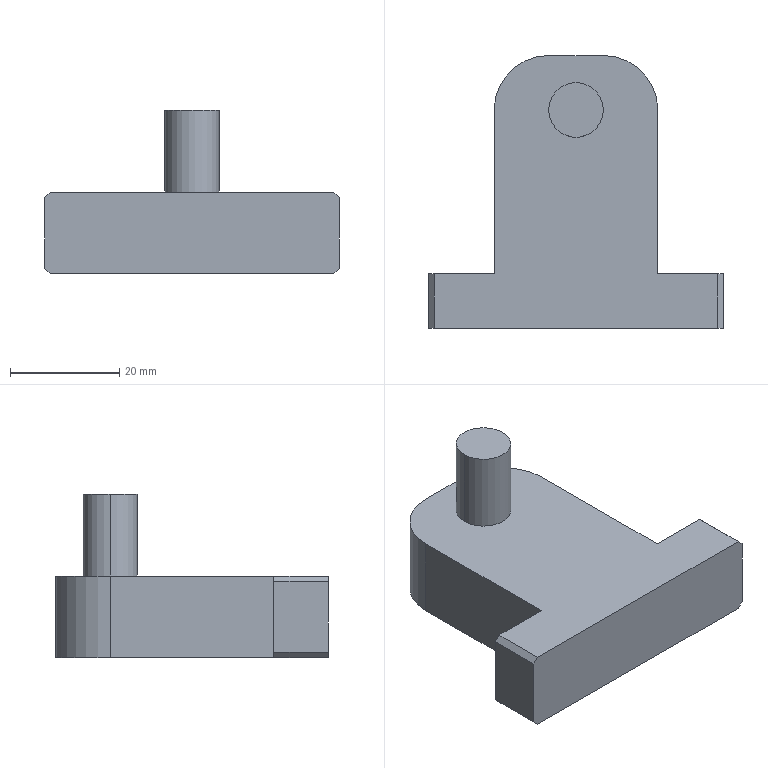Part | SolidWorks | 1 solid | 19 faces | box 54 x 50 x 30 mm | volume 26614 mm3 | plane 15 | cylinder 4 | commonest cylinder face diameters 10 x2 20 x2
STEP:
#1=CARTESIAN_POINT('',(5.,35.,30.));
#2=VERTEX_POINT('',#1);
#3=CARTESIAN_POINT('',(-5.,35.,30.));
#4=VERTEX_POINT('',#3);
#5=CARTESIAN_POINT('',(0.,35.,30.));
#6=DIRECTION('',(0.,0.,1.));
#7=DIRECTION('',(1.,0.,0.));
#8=AXIS2_PLACEMENT_3D('',#5,#6,#7);
#9=CIRCLE('',#8,5.);
#10=EDGE_CURVE('',#2,#4,#9,.T.);
#11=ORIENTED_EDGE('',*,*,#10,.F.);
#12=CARTESIAN_POINT('',(5.,35.,15.));
#13=VERTEX_POINT('',#12);
#14=CARTESIAN_POINT('',(5.,35.,30.));
#15=DIRECTION('',(0.,0.,-1.));
#16=VECTOR('',#15,1000.);
#17=LINE('',#14,#16);
#18=EDGE_CURVE('',#2,#13,#17,.T.);
#19=ORIENTED_EDGE('',*,*,#18,.T.);
#20=CARTESIAN_POINT('',(-5.,35.,15.));
#21=VERTEX_POINT('',#20);
#22=CARTESIAN_POINT('',(0.,35.,15.));
#23=DIRECTION('',(0.,0.,1.));
#24=DIRECTION('',(1.,0.,0.));
#25=AXIS2_PLACEMENT_3D('',#22,#23,#24);
#26=CIRCLE('',#25,5.);
#27=EDGE_CURVE('',#13,#21,#26,.T.);
#28=ORIENTED_EDGE('',*,*,#27,.T.);
#29=CARTESIAN_POINT('',(-5.,35.,30.));
#30=DIRECTION('',(0.,0.,-1.));
#31=VECTOR('',#30,1000.);
#32=LINE('',#29,#31);
#33=EDGE_CURVE('',#4,#21,#32,.T.);
#34=ORIENTED_EDGE('',*,*,#33,.F.);
#35=EDGE_LOOP('',(#11,#19,#28,#34));
#36=FACE_OUTER_BOUND('',#35,.T.);
#37=CARTESIAN_POINT('',(0.,35.,30.));
#38=DIRECTION('',(0.,0.,-1.));
#39=DIRECTION('',(-1.,0.,0.));
#40=AXIS2_PLACEMENT_3D('',#37,#38,#39);
#41=CYLINDRICAL_SURFACE('',#40,5.);
#42=ADVANCED_FACE('',(#36),#41,.T.);
#43=CARTESIAN_POINT('',(27.,-5.,14.));
#44=VERTEX_POINT('',#43);
#45=CARTESIAN_POINT('',(27.,-5.,1.));
#46=VERTEX_POINT('',#45);
#47=CARTESIAN_POINT('',(27.,-5.,15.));
#48=DIRECTION('',(0.,0.,-1.));
#49=VECTOR('',#48,1000.);
#50=LINE('',#47,#49);
#51=EDGE_CURVE('',#44,#46,#50,.T.);
#52=ORIENTED_EDGE('',*,*,#51,.T.);
#53=CARTESIAN_POINT('',(27.,5.,1.));
#54=VERTEX_POINT('',#53);
#55=CARTESIAN_POINT('',(27.,5.,1.));
#56=DIRECTION('',(0.,1.,0.));
#57=VECTOR('',#56,1000.);
#58=LINE('',#55,#57);
#59=EDGE_CURVE('',#46,#54,#58,.T.);
#60=ORIENTED_EDGE('',*,*,#59,.T.);
#61=CARTESIAN_POINT('',(27.,5.,14.));
#62=VERTEX_POINT('',#61);
#63=CARTESIAN_POINT('',(27.,5.,15.));
#64=DIRECTION('',(0.,0.,-1.));
#65=VECTOR('',#64,1000.);
#66=LINE('',#63,#65);
#67=EDGE_CURVE('',#62,#54,#66,.T.);
#68=ORIENTED_EDGE('',*,*,#67,.F.);
#69=CARTESIAN_POINT('',(27.,-5.,14.));
#70=DIRECTION('',(0.,-1.,0.));
#71=VECTOR('',#70,1000.);
#72=LINE('',#69,#71);
#73=EDGE_CURVE('',#62,#44,#72,.T.);
#74=ORIENTED_EDGE('',*,*,#73,.T.);
#75=EDGE_LOOP('',(#52,#60,#68,#74));
#76=FACE_OUTER_BOUND('',#75,.T.);
#77=CARTESIAN_POINT('',(27.,5.,15.));
#78=DIRECTION('',(-1.,0.,0.));
#79=DIRECTION('',(0.,-1.,0.));
#80=AXIS2_PLACEMENT_3D('',#77,#78,#79);
#81=PLANE('',#80);
#82=ADVANCED_FACE('',(#76),#81,.F.);
#83=ORIENTED_EDGE('',*,*,#67,.T.);
#84=CARTESIAN_POINT('',(26.,5.,0.));
#85=VERTEX_POINT('',#84);
#86=CARTESIAN_POINT('',(27.,5.,1.));
#87=DIRECTION('',(-0.7071,0.,-0.7071));
#88=VECTOR('',#87,1000.);
#89=LINE('',#86,#88);
#90=EDGE_CURVE('',#54,#85,#89,.T.);
#91=ORIENTED_EDGE('',*,*,#90,.T.);
#92=CARTESIAN_POINT('',(15.,5.,0.));
#93=VERTEX_POINT('',#92);
#94=CARTESIAN_POINT('',(15.,5.,0.));
#95=DIRECTION('',(-1.,0.,0.));
#96=VECTOR('',#95,1000.);
#97=LINE('',#94,#96);
#98=EDGE_CURVE('',#85,#93,#97,.T.);
#99=ORIENTED_EDGE('',*,*,#98,.T.);
#100=CARTESIAN_POINT('',(15.,5.,15.));
#101=VERTEX_POINT('',#100);
#102=CARTESIAN_POINT('',(15.,5.,15.));
#103=DIRECTION('',(0.,0.,-1.));
#104=VECTOR('',#103,1000.);
#105=LINE('',#102,#104);
#106=EDGE_CURVE('',#101,#93,#105,.T.);
#107=ORIENTED_EDGE('',*,*,#106,.F.);
#108=CARTESIAN_POINT('',(26.,5.,15.));
#109=VERTEX_POINT('',#108);
#110=CARTESIAN_POINT('',(15.,5.,15.));
#111=DIRECTION('',(-1.,0.,0.));
#112=VECTOR('',#111,1000.);
#113=LINE('',#110,#112);
#114=EDGE_CURVE('',#109,#101,#113,.T.);
#115=ORIENTED_EDGE('',*,*,#114,.F.);
#116=CARTESIAN_POINT('',(26.,5.,15.));
#117=DIRECTION('',(0.7071,0.,-0.7071));
#118=VECTOR('',#117,1000.);
#119=LINE('',#116,#118);
#120=EDGE_CURVE('',#109,#62,#119,.T.);
#121=ORIENTED_EDGE('',*,*,#120,.T.);
#122=EDGE_LOOP('',(#83,#91,#99,#107,#115,#121));
#123=FACE_OUTER_BOUND('',#122,.T.);
#124=CARTESIAN_POINT('',(15.,5.,15.));
#125=DIRECTION('',(0.,-1.,0.));
#126=DIRECTION('',(0.,0.,-1.));
#127=AXIS2_PLACEMENT_3D('',#124,#125,#126);
#128=PLANE('',#127);
#129=ADVANCED_FACE('',(#123),#128,.F.);
#130=CARTESIAN_POINT('',(15.,35.,0.));
#131=VERTEX_POINT('',#130);
#132=CARTESIAN_POINT('',(15.,5.,0.));
#133=DIRECTION('',(0.,1.,0.));
#134=VECTOR('',#133,1000.);
#135=LINE('',#132,#134);
#136=EDGE_CURVE('',#93,#131,#135,.T.);
#137=ORIENTED_EDGE('',*,*,#136,.T.);
#138=CARTESIAN_POINT('',(15.,35.,15.));
#139=VERTEX_POINT('',#138);
#140=CARTESIAN_POINT('',(15.,35.,15.));
#141=DIRECTION('',(0.,0.,1.));
#142=VECTOR('',#141,1000.);
#143=LINE('',#140,#142);
#144=EDGE_CURVE('',#131,#139,#143,.T.);
#145=ORIENTED_EDGE('',*,*,#144,.T.);
#146=CARTESIAN_POINT('',(15.,5.,15.));
#147=DIRECTION('',(0.,1.,0.));
#148=VECTOR('',#147,1000.);
#149=LINE('',#146,#148);
#150=EDGE_CURVE('',#101,#139,#149,.T.);
#151=ORIENTED_EDGE('',*,*,#150,.F.);
#152=ORIENTED_EDGE('',*,*,#106,.T.);
#153=EDGE_LOOP('',(#137,#145,#151,#152));
#154=FACE_OUTER_BOUND('',#153,.T.);
#155=CARTESIAN_POINT('',(15.,5.,15.));
#156=DIRECTION('',(-1.,0.,0.));
#157=DIRECTION('',(0.,-1.,0.));
#158=AXIS2_PLACEMENT_3D('',#155,#156,#157);
#159=PLANE('',#158);
#160=ADVANCED_FACE('',(#154),#159,.F.);
#161=CARTESIAN_POINT('',(5.,45.,0.));
#162=VERTEX_POINT('',#161);
#163=CARTESIAN_POINT('',(-5.,45.,0.));
#164=VERTEX_POINT('',#163);
#165=CARTESIAN_POINT('',(-15.,45.,0.));
#166=DIRECTION('',(-1.,0.,0.));
#167=VECTOR('',#166,1000.);
#168=LINE('',#165,#167);
#169=EDGE_CURVE('',#162,#164,#168,.T.);
#170=ORIENTED_EDGE('',*,*,#169,.T.);
#171=CARTESIAN_POINT('',(-5.,45.,15.));
#172=VERTEX_POINT('',#171);
#173=CARTESIAN_POINT('',(-5.,45.,15.));
#174=DIRECTION('',(0.,0.,1.));
#175=VECTOR('',#174,1000.);
#176=LINE('',#173,#175);
#177=EDGE_CURVE('',#164,#172,#176,.T.);
#178=ORIENTED_EDGE('',*,*,#177,.T.);
#179=CARTESIAN_POINT('',(5.,45.,15.));
#180=VERTEX_POINT('',#179);
#181=CARTESIAN_POINT('',(-15.,45.,15.));
#182=DIRECTION('',(-1.,0.,0.));
#183=VECTOR('',#182,1000.);
#184=LINE('',#181,#183);
#185=EDGE_CURVE('',#180,#172,#184,.T.);
#186=ORIENTED_EDGE('',*,*,#185,.F.);
#187=CARTESIAN_POINT('',(5.,45.,15.));
#188=DIRECTION('',(0.,0.,-1.));
#189=VECTOR('',#188,1000.);
#190=LINE('',#187,#189);
#191=EDGE_CURVE('',#180,#162,#190,.T.);
#192=ORIENTED_EDGE('',*,*,#191,.T.);
#193=EDGE_LOOP('',(#170,#178,#186,#192));
#194=FACE_OUTER_BOUND('',#193,.T.);
#195=CARTESIAN_POINT('',(-15.,45.,15.));
#196=DIRECTION('',(0.,-1.,0.));
#197=DIRECTION('',(0.,0.,-1.));
#198=AXIS2_PLACEMENT_3D('',#195,#196,#197);
#199=PLANE('',#198);
#200=ADVANCED_FACE('',(#194),#199,.F.);
#201=CARTESIAN_POINT('',(-15.,35.,15.));
#202=VERTEX_POINT('',#201);
#203=CARTESIAN_POINT('',(-15.,5.,15.));
#204=VERTEX_POINT('',#203);
#205=CARTESIAN_POINT('',(-15.,5.,15.));
#206=DIRECTION('',(0.,-1.,0.));
#207=VECTOR('',#206,1000.);
#208=LINE('',#205,#207);
#209=EDGE_CURVE('',#202,#204,#208,.T.);
#210=ORIENTED_EDGE('',*,*,#209,.F.);
#211=CARTESIAN_POINT('',(-15.,35.,0.));
#212=VERTEX_POINT('',#211);
#213=CARTESIAN_POINT('',(-15.,35.,15.));
#214=DIRECTION('',(0.,0.,-1.));
#215=VECTOR('',#214,1000.);
#216=LINE('',#213,#215);
#217=EDGE_CURVE('',#202,#212,#216,.T.);
#218=ORIENTED_EDGE('',*,*,#217,.T.);
#219=CARTESIAN_POINT('',(-15.,5.,0.));
#220=VERTEX_POINT('',#219);
#221=CARTESIAN_POINT('',(-15.,5.,0.));
#222=DIRECTION('',(0.,-1.,0.));
#223=VECTOR('',#222,1000.);
#224=LINE('',#221,#223);
#225=EDGE_CURVE('',#212,#220,#224,.T.);
#226=ORIENTED_EDGE('',*,*,#225,.T.);
#227=CARTESIAN_POINT('',(-15.,5.,15.));
#228=DIRECTION('',(0.,0.,-1.));
#229=VECTOR('',#228,1000.);
#230=LINE('',#227,#229);
#231=EDGE_CURVE('',#204,#220,#230,.T.);
#232=ORIENTED_EDGE('',*,*,#231,.F.);
#233=EDGE_LOOP('',(#210,#218,#226,#232));
#234=FACE_OUTER_BOUND('',#233,.T.);
#235=CARTESIAN_POINT('',(-15.,5.,15.));
#236=DIRECTION('',(1.,0.,0.));
#237=DIRECTION('',(0.,1.,0.));
#238=AXIS2_PLACEMENT_3D('',#235,#236,#237);
#239=PLANE('',#238);
#240=ADVANCED_FACE('',(#234),#239,.F.);
#241=CARTESIAN_POINT('',(-27.,5.,14.));
#242=VERTEX_POINT('',#241);
#243=CARTESIAN_POINT('',(-27.,5.,1.));
#244=VERTEX_POINT('',#243);
#245=CARTESIAN_POINT('',(-27.,5.,15.));
#246=DIRECTION('',(0.,0.,-1.));
#247=VECTOR('',#246,1000.);
#248=LINE('',#245,#247);
#249=EDGE_CURVE('',#242,#244,#248,.T.);
#250=ORIENTED_EDGE('',*,*,#249,.F.);
#251=CARTESIAN_POINT('',(-26.,5.,15.));
#252=VERTEX_POINT('',#251);
#253=CARTESIAN_POINT('',(-26.,5.,15.));
#254=DIRECTION('',(0.7071,0.,0.7071));
#255=VECTOR('',#254,1000.);
#256=LINE('',#253,#255);
#257=EDGE_CURVE('',#242,#252,#256,.T.);
#258=ORIENTED_EDGE('',*,*,#257,.T.);
#259=CARTESIAN_POINT('',(-27.,5.,15.));
#260=DIRECTION('',(-1.,0.,0.));
#261=VECTOR('',#260,1000.);
#262=LINE('',#259,#261);
#263=EDGE_CURVE('',#204,#252,#262,.T.);
#264=ORIENTED_EDGE('',*,*,#263,.F.);
#265=ORIENTED_EDGE('',*,*,#231,.T.);
#266=CARTESIAN_POINT('',(-26.,5.,0.));
#267=VERTEX_POINT('',#266);
#268=CARTESIAN_POINT('',(-27.,5.,0.));
#269=DIRECTION('',(-1.,0.,0.));
#270=VECTOR('',#269,1000.);
#271=LINE('',#268,#270);
#272=EDGE_CURVE('',#220,#267,#271,.T.);
#273=ORIENTED_EDGE('',*,*,#272,.T.);
#274=CARTESIAN_POINT('',(-27.,5.,1.));
#275=DIRECTION('',(-0.7071,0.,0.7071));
#276=VECTOR('',#275,1000.);
#277=LINE('',#274,#276);
#278=EDGE_CURVE('',#267,#244,#277,.T.);
#279=ORIENTED_EDGE('',*,*,#278,.T.);
#280=EDGE_LOOP('',(#250,#258,#264,#265,#273,#279));
#281=FACE_OUTER_BOUND('',#280,.T.);
#282=CARTESIAN_POINT('',(-27.,5.,15.));
#283=DIRECTION('',(0.,-1.,0.));
#284=DIRECTION('',(0.,0.,-1.));
#285=AXIS2_PLACEMENT_3D('',#282,#283,#284);
#286=PLANE('',#285);
#287=ADVANCED_FACE('',(#281),#286,.F.);
#288=CARTESIAN_POINT('',(-27.,-5.,14.));
#289=VERTEX_POINT('',#288);
#290=CARTESIAN_POINT('',(-27.,-5.,1.));
#291=VERTEX_POINT('',#290);
#292=CARTESIAN_POINT('',(-27.,-5.,15.));
#293=DIRECTION('',(0.,0.,-1.));
#294=VECTOR('',#293,1000.);
#295=LINE('',#292,#294);
#296=EDGE_CURVE('',#289,#291,#295,.T.);
#297=ORIENTED_EDGE('',*,*,#296,.F.);
#298=CARTESIAN_POINT('',(-27.,5.,14.));
#299=DIRECTION('',(0.,1.,0.));
#300=VECTOR('',#299,1000.);
#301=LINE('',#298,#300);
#302=EDGE_CURVE('',#289,#242,#301,.T.);
#303=ORIENTED_EDGE('',*,*,#302,.T.);
#304=ORIENTED_EDGE('',*,*,#249,.T.);
#305=CARTESIAN_POINT('',(-27.,5.,1.));
#306=DIRECTION('',(0.,-1.,0.));
#307=VECTOR('',#306,1000.);
#308=LINE('',#305,#307);
#309=EDGE_CURVE('',#244,#291,#308,.T.);
#310=ORIENTED_EDGE('',*,*,#309,.T.);
#311=EDGE_LOOP('',(#297,#303,#304,#310));
#312=FACE_OUTER_BOUND('',#311,.T.);
#313=CARTESIAN_POINT('',(-27.,5.,15.));
#314=DIRECTION('',(1.,0.,0.));
#315=DIRECTION('',(0.,1.,0.));
#316=AXIS2_PLACEMENT_3D('',#313,#314,#315);
#317=PLANE('',#316);
#318=ADVANCED_FACE('',(#312),#317,.F.);
#319=CARTESIAN_POINT('',(-26.,-5.,0.));
#320=VERTEX_POINT('',#319);
#321=CARTESIAN_POINT('',(26.,-5.,0.));
#322=VERTEX_POINT('',#321);
#323=CARTESIAN_POINT('',(-27.,-5.,0.));
#324=DIRECTION('',(1.,0.,0.));
#325=VECTOR('',#324,1000.);
#326=LINE('',#323,#325);
#327=EDGE_CURVE('',#320,#322,#326,.T.);
#328=ORIENTED_EDGE('',*,*,#327,.T.);
#329=CARTESIAN_POINT('',(27.,-5.,1.));
#330=DIRECTION('',(0.7071,0.,0.7071));
#331=VECTOR('',#330,1000.);
#332=LINE('',#329,#331);
#333=EDGE_CURVE('',#322,#46,#332,.T.);
#334=ORIENTED_EDGE('',*,*,#333,.T.);
#335=ORIENTED_EDGE('',*,*,#51,.F.);
#336=CARTESIAN_POINT('',(26.,-5.,15.));
#337=VERTEX_POINT('',#336);
#338=CARTESIAN_POINT('',(26.,-5.,15.));
#339=DIRECTION('',(-0.7071,0.,0.7071));
#340=VECTOR('',#339,1000.);
#341=LINE('',#338,#340);
#342=EDGE_CURVE('',#44,#337,#341,.T.);
#343=ORIENTED_EDGE('',*,*,#342,.T.);
#344=CARTESIAN_POINT('',(-26.,-5.,15.));
#345=VERTEX_POINT('',#344);
#346=CARTESIAN_POINT('',(-27.,-5.,15.));
#347=DIRECTION('',(1.,0.,0.));
#348=VECTOR('',#347,1000.);
#349=LINE('',#346,#348);
#350=EDGE_CURVE('',#345,#337,#349,.T.);
#351=ORIENTED_EDGE('',*,*,#350,.F.);
#352=CARTESIAN_POINT('',(-26.,-5.,15.));
#353=DIRECTION('',(-0.7071,0.,-0.7071));
#354=VECTOR('',#353,1000.);
#355=LINE('',#352,#354);
#356=EDGE_CURVE('',#345,#289,#355,.T.);
#357=ORIENTED_EDGE('',*,*,#356,.T.);
#358=ORIENTED_EDGE('',*,*,#296,.T.);
#359=CARTESIAN_POINT('',(-27.,-5.,1.));
#360=DIRECTION('',(0.7071,0.,-0.7071));
#361=VECTOR('',#360,1000.);
#362=LINE('',#359,#361);
#363=EDGE_CURVE('',#291,#320,#362,.T.);
#364=ORIENTED_EDGE('',*,*,#363,.T.);
#365=EDGE_LOOP('',(#328,#334,#335,#343,#351,#357,#358,#364));
#366=FACE_OUTER_BOUND('',#365,.T.);
#367=CARTESIAN_POINT('',(-27.,-5.,15.));
#368=DIRECTION('',(0.,1.,0.));
#369=DIRECTION('',(0.,0.,1.));
#370=AXIS2_PLACEMENT_3D('',#367,#368,#369);
#371=PLANE('',#370);
#372=ADVANCED_FACE('',(#366),#371,.F.);
#373=CARTESIAN_POINT('',(0.,35.,15.));
#374=DIRECTION('',(0.,0.,1.));
#375=DIRECTION('',(1.,0.,0.));
#376=AXIS2_PLACEMENT_3D('',#373,#374,#375);
#377=CIRCLE('',#376,5.);
#378=EDGE_CURVE('',#21,#13,#377,.T.);
#379=ORIENTED_EDGE('',*,*,#378,.F.);
#380=ORIENTED_EDGE('',*,*,#27,.F.);
#381=EDGE_LOOP('',(#379,#380));
#382=FACE_BOUND('',#381,.T.);
#383=ORIENTED_EDGE('',*,*,#350,.T.);
#384=CARTESIAN_POINT('',(26.,5.,15.));
#385=DIRECTION('',(0.,1.,0.));
#386=VECTOR('',#385,1000.);
#387=LINE('',#384,#386);
#388=EDGE_CURVE('',#337,#109,#387,.T.);
#389=ORIENTED_EDGE('',*,*,#388,.T.);
#390=ORIENTED_EDGE('',*,*,#114,.T.);
#391=ORIENTED_EDGE('',*,*,#150,.T.);
#392=CARTESIAN_POINT('',(5.,35.,15.));
#393=DIRECTION('',(0.,0.,1.));
#394=DIRECTION('',(1.,0.,0.));
#395=AXIS2_PLACEMENT_3D('',#392,#393,#394);
#396=CIRCLE('',#395,10.);
#397=EDGE_CURVE('',#139,#180,#396,.T.);
#398=ORIENTED_EDGE('',*,*,#397,.T.);
#399=ORIENTED_EDGE('',*,*,#185,.T.);
#400=CARTESIAN_POINT('',(-5.,35.,15.));
#401=DIRECTION('',(0.,0.,1.));
#402=DIRECTION('',(1.,0.,0.));
#403=AXIS2_PLACEMENT_3D('',#400,#401,#402);
#404=CIRCLE('',#403,10.);
#405=EDGE_CURVE('',#172,#202,#404,.T.);
#406=ORIENTED_EDGE('',*,*,#405,.T.);
#407=ORIENTED_EDGE('',*,*,#209,.T.);
#408=ORIENTED_EDGE('',*,*,#263,.T.);
#409=CARTESIAN_POINT('',(-26.,-5.,15.));
#410=DIRECTION('',(0.,-1.,0.));
#411=VECTOR('',#410,1000.);
#412=LINE('',#409,#411);
#413=EDGE_CURVE('',#252,#345,#412,.T.);
#414=ORIENTED_EDGE('',*,*,#413,.T.);
#415=EDGE_LOOP('',(#383,#389,#390,#391,#398,#399,#406,#407,#408,#414));
#416=FACE_OUTER_BOUND('',#415,.T.);
#417=CARTESIAN_POINT('',(0.,0.,15.));
#418=DIRECTION('',(0.,0.,1.));
#419=DIRECTION('',(1.,0.,0.));
#420=AXIS2_PLACEMENT_3D('',#417,#418,#419);
#421=PLANE('',#420);
#422=ADVANCED_FACE('',(#382,#416),#421,.T.);
#423=ORIENTED_EDGE('',*,*,#98,.F.);
#424=CARTESIAN_POINT('',(26.,0.,0.));
#425=DIRECTION('',(0.,-1.,0.));
#426=VECTOR('',#425,1000.);
#427=LINE('',#424,#426);
#428=EDGE_CURVE('',#85,#322,#427,.T.);
#429=ORIENTED_EDGE('',*,*,#428,.T.);
#430=ORIENTED_EDGE('',*,*,#327,.F.);
#431=CARTESIAN_POINT('',(-26.,0.,0.));
#432=DIRECTION('',(0.,1.,0.));
#433=VECTOR('',#432,1000.);
#434=LINE('',#431,#433);
#435=EDGE_CURVE('',#320,#267,#434,.T.);
#436=ORIENTED_EDGE('',*,*,#435,.T.);
#437=ORIENTED_EDGE('',*,*,#272,.F.);
#438=ORIENTED_EDGE('',*,*,#225,.F.);
#439=CARTESIAN_POINT('',(-5.,35.,0.));
#440=DIRECTION('',(0.,0.,-1.));
#441=DIRECTION('',(1.,0.,0.));
#442=AXIS2_PLACEMENT_3D('',#439,#440,#441);
#443=CIRCLE('',#442,10.);
#444=EDGE_CURVE('',#212,#164,#443,.T.);
#445=ORIENTED_EDGE('',*,*,#444,.T.);
#446=ORIENTED_EDGE('',*,*,#169,.F.);
#447=CARTESIAN_POINT('',(5.,35.,0.));
#448=DIRECTION('',(0.,0.,-1.));
#449=DIRECTION('',(1.,0.,0.));
#450=AXIS2_PLACEMENT_3D('',#447,#448,#449);
#451=CIRCLE('',#450,10.);
#452=EDGE_CURVE('',#162,#131,#451,.T.);
#453=ORIENTED_EDGE('',*,*,#452,.T.);
#454=ORIENTED_EDGE('',*,*,#136,.F.);
#455=EDGE_LOOP('',(#423,#429,#430,#436,#437,#438,#445,#446,#453,#454));
#456=FACE_OUTER_BOUND('',#455,.T.);
#457=CARTESIAN_POINT('',(0.,0.,0.));
#458=DIRECTION('',(0.,0.,1.));
#459=DIRECTION('',(1.,0.,0.));
#460=AXIS2_PLACEMENT_3D('',#457,#458,#459);
#461=PLANE('',#460);
#462=ADVANCED_FACE('',(#456),#461,.F.);
#463=ORIENTED_EDGE('',*,*,#405,.F.);
#464=ORIENTED_EDGE('',*,*,#177,.F.);
#465=ORIENTED_EDGE('',*,*,#444,.F.);
#466=ORIENTED_EDGE('',*,*,#217,.F.);
#467=EDGE_LOOP('',(#463,#464,#465,#466));
#468=FACE_OUTER_BOUND('',#467,.T.);
#469=CARTESIAN_POINT('',(-5.,35.,15.));
#470=DIRECTION('',(0.,0.,-1.));
#471=DIRECTION('',(-1.,0.,0.));
#472=AXIS2_PLACEMENT_3D('',#469,#470,#471);
#473=CYLINDRICAL_SURFACE('',#472,10.);
#474=ADVANCED_FACE('',(#468),#473,.T.);
#475=ORIENTED_EDGE('',*,*,#397,.F.);
#476=ORIENTED_EDGE('',*,*,#144,.F.);
#477=ORIENTED_EDGE('',*,*,#452,.F.);
#478=ORIENTED_EDGE('',*,*,#191,.F.);
#479=EDGE_LOOP('',(#475,#476,#477,#478));
#480=FACE_OUTER_BOUND('',#479,.T.);
#481=CARTESIAN_POINT('',(5.,35.,15.));
#482=DIRECTION('',(0.,0.,-1.));
#483=DIRECTION('',(-1.,0.,0.));
#484=AXIS2_PLACEMENT_3D('',#481,#482,#483);
#485=CYLINDRICAL_SURFACE('',#484,10.);
#486=ADVANCED_FACE('',(#480),#485,.T.);
#487=ORIENTED_EDGE('',*,*,#18,.F.);
#488=CARTESIAN_POINT('',(0.,35.,30.));
#489=DIRECTION('',(0.,0.,1.));
#490=DIRECTION('',(1.,0.,0.));
#491=AXIS2_PLACEMENT_3D('',#488,#489,#490);
#492=CIRCLE('',#491,5.);
#493=EDGE_CURVE('',#4,#2,#492,.T.);
#494=ORIENTED_EDGE('',*,*,#493,.F.);
#495=ORIENTED_EDGE('',*,*,#33,.T.);
#496=ORIENTED_EDGE('',*,*,#378,.T.);
#497=EDGE_LOOP('',(#487,#494,#495,#496));
#498=FACE_OUTER_BOUND('',#497,.T.);
#499=CARTESIAN_POINT('',(0.,35.,30.));
#500=DIRECTION('',(0.,0.,-1.));
#501=DIRECTION('',(-1.,0.,0.));
#502=AXIS2_PLACEMENT_3D('',#499,#500,#501);
#503=CYLINDRICAL_SURFACE('',#502,5.);
#504=ADVANCED_FACE('',(#498),#503,.T.);
#505=ORIENTED_EDGE('',*,*,#493,.T.);
#506=ORIENTED_EDGE('',*,*,#10,.T.);
#507=EDGE_LOOP('',(#505,#506));
#508=FACE_OUTER_BOUND('',#507,.T.);
#509=CARTESIAN_POINT('',(0.,35.,30.));
#510=DIRECTION('',(0.,0.,1.));
#511=DIRECTION('',(1.,0.,0.));
#512=AXIS2_PLACEMENT_3D('',#509,#510,#511);
#513=PLANE('',#512);
#514=ADVANCED_FACE('',(#508),#513,.T.);
#515=ORIENTED_EDGE('',*,*,#333,.F.);
#516=ORIENTED_EDGE('',*,*,#428,.F.);
#517=ORIENTED_EDGE('',*,*,#90,.F.);
#518=ORIENTED_EDGE('',*,*,#59,.F.);
#519=EDGE_LOOP('',(#515,#516,#517,#518));
#520=FACE_OUTER_BOUND('',#519,.T.);
#521=CARTESIAN_POINT('',(27.,5.,1.));
#522=DIRECTION('',(-0.7071,0.,0.7071));
#523=DIRECTION('',(0.,1.,0.));
#524=AXIS2_PLACEMENT_3D('',#521,#522,#523);
#525=PLANE('',#524);
#526=ADVANCED_FACE('',(#520),#525,.F.);
#527=ORIENTED_EDGE('',*,*,#342,.F.);
#528=ORIENTED_EDGE('',*,*,#73,.F.);
#529=ORIENTED_EDGE('',*,*,#120,.F.);
#530=ORIENTED_EDGE('',*,*,#388,.F.);
#531=EDGE_LOOP('',(#527,#528,#529,#530));
#532=FACE_OUTER_BOUND('',#531,.T.);
#533=CARTESIAN_POINT('',(26.,0.,15.));
#534=DIRECTION('',(0.7071,0.,0.7071));
#535=DIRECTION('',(0.,-1.,0.));
#536=AXIS2_PLACEMENT_3D('',#533,#534,#535);
#537=PLANE('',#536);
#538=ADVANCED_FACE('',(#532),#537,.T.);
#539=ORIENTED_EDGE('',*,*,#257,.F.);
#540=ORIENTED_EDGE('',*,*,#302,.F.);
#541=ORIENTED_EDGE('',*,*,#356,.F.);
#542=ORIENTED_EDGE('',*,*,#413,.F.);
#543=EDGE_LOOP('',(#539,#540,#541,#542));
#544=FACE_OUTER_BOUND('',#543,.T.);
#545=CARTESIAN_POINT('',(-26.,0.,15.));
#546=DIRECTION('',(-0.7071,0.,0.7071));
#547=DIRECTION('',(0.,1.,0.));
#548=AXIS2_PLACEMENT_3D('',#545,#546,#547);
#549=PLANE('',#548);
#550=ADVANCED_FACE('',(#544),#549,.T.);
#551=ORIENTED_EDGE('',*,*,#278,.F.);
#552=ORIENTED_EDGE('',*,*,#435,.F.);
#553=ORIENTED_EDGE('',*,*,#363,.F.);
#554=ORIENTED_EDGE('',*,*,#309,.F.);
#555=EDGE_LOOP('',(#551,#552,#553,#554));
#556=FACE_OUTER_BOUND('',#555,.T.);
#557=CARTESIAN_POINT('',(-27.,5.,1.));
#558=DIRECTION('',(0.7071,0.,0.7071));
#559=DIRECTION('',(0.,-1.,0.));
#560=AXIS2_PLACEMENT_3D('',#557,#558,#559);
#561=PLANE('',#560);
#562=ADVANCED_FACE('',(#556),#561,.F.);
#563=CLOSED_SHELL('',(#42,#82,#129,#160,#200,#240,#287,#318,#372,#422,#462,#474,#486,#504,#514,#526,#538,#550,#562));
#564=MANIFOLD_SOLID_BREP('',#563);
#565=CARTESIAN_POINT('',(0.,0.,0.));
#566=DIRECTION('',(0.,0.,1.));
#567=DIRECTION('',(1.,0.,0.));
#568=AXIS2_PLACEMENT_3D('',#565,#566,#567);
#569=(LENGTH_UNIT()NAMED_UNIT(*)SI_UNIT(.MILLI.,.METRE.));
#570=UNCERTAINTY_MEASURE_WITH_UNIT(LENGTH_MEASURE(0.00001),#569,'','');
#571=(NAMED_UNIT(*)PLANE_ANGLE_UNIT()SI_UNIT($,.RADIAN.));
#572=(NAMED_UNIT(*)SI_UNIT($,.STERADIAN.)SOLID_ANGLE_UNIT());
#573=(GEOMETRIC_REPRESENTATION_CONTEXT(3)GLOBAL_UNCERTAINTY_ASSIGNED_CONTEXT((#570))GLOBAL_UNIT_ASSIGNED_CONTEXT((#569,#571,#572))REPRESENTATION_CONTEXT('',''));
#574=ADVANCED_BREP_SHAPE_REPRESENTATION('',(#564,#568),#573);